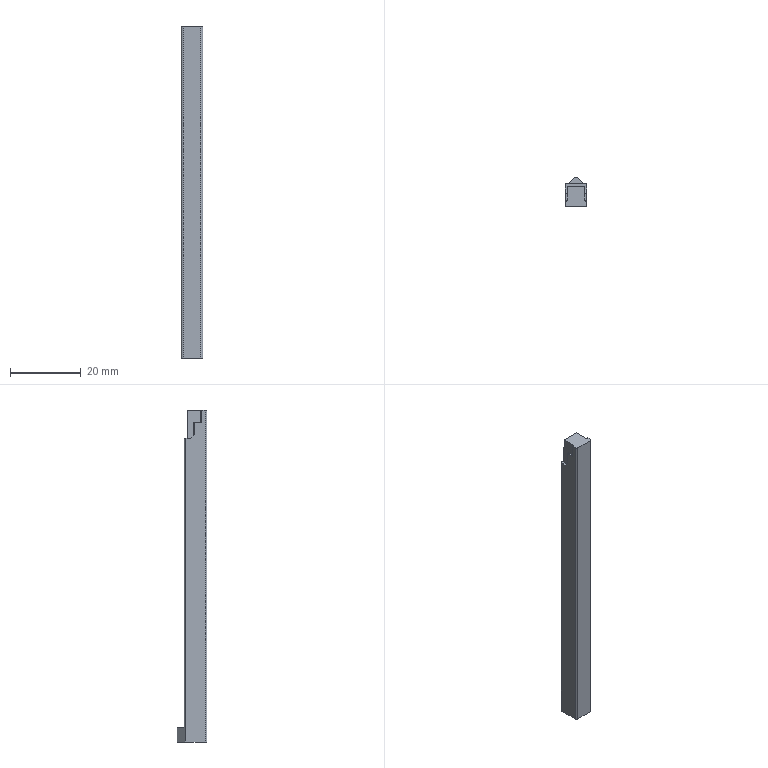Part | Creo | 1 solid | 30 faces | box 6.096 x 8.5 x 94.171 mm | volume 3667 mm3 | plane 22 | cylinder 8 | commonest cylinder face diameters 0.603 x4 1 x4
STEP:
#1=CARTESIAN_POINT('',(0.,0.,0.));
#2=DIRECTION('',(0.,0.,1.));
#3=DIRECTION('',(1.,0.,0.));
#4=AXIS2_PLACEMENT_3D('',#1,#2,#3);
#5=CARTESIAN_POINT('',(-2.088,17.979,36.563));
#6=VERTEX_POINT('',#5);
#7=CARTESIAN_POINT('',(-1.787,17.677,36.563));
#8=VERTEX_POINT('',#7);
#9=CARTESIAN_POINT('',(-2.088,17.878,36.563));
#10=CARTESIAN_POINT('',(-2.012,17.754,36.563));
#11=CARTESIAN_POINT('',(-1.887,17.677,36.563));
#12=B_SPLINE_CURVE_WITH_KNOTS('',3,(#5,#9,#10,#11,#7),.UNSPECIFIED.,.F.,.F.,(4,1,4),(0.,0.5,1.),.UNSPECIFIED.);
#13=EDGE_CURVE('',#6,#8,#12,.T.);
#14=ORIENTED_EDGE('',*,*,#13,.F.);
#15=CARTESIAN_POINT('',(-2.055,18.012,32.744));
#16=VERTEX_POINT('',#15);
#17=CARTESIAN_POINT('',(-2.088,17.979,36.563));
#18=DIRECTION('',(0.008726,0.008726,-0.9999));
#19=VECTOR('',#18,3.819);
#20=LINE('',#17,#19);
#21=EDGE_CURVE('',#6,#16,#20,.T.);
#22=ORIENTED_EDGE('',*,*,#21,.T.);
#23=CARTESIAN_POINT('',(-1.757,17.708,33.046));
#24=VERTEX_POINT('',#23);
#25=CARTESIAN_POINT('',(-1.757,17.708,33.046));
#26=CARTESIAN_POINT('',(-1.788,17.708,33.046));
#27=CARTESIAN_POINT('',(-1.849,17.718,33.036));
#28=CARTESIAN_POINT('',(-1.934,17.761,32.993));
#29=CARTESIAN_POINT('',(-1.999,17.826,32.929));
#30=CARTESIAN_POINT('',(-2.044,17.911,32.845));
#31=CARTESIAN_POINT('',(-2.055,17.977,32.78));
#32=B_SPLINE_CURVE_WITH_KNOTS('',3,(#25,#26,#27,#28,#29,#30,#31,#15),.UNSPECIFIED.,.F.,.F.,(4,1,1,1,1,4),(0.,0.2,0.4,0.6,0.8,1.),.UNSPECIFIED.);
#33=EDGE_CURVE('',#24,#16,#32,.T.);
#34=ORIENTED_EDGE('',*,*,#33,.F.);
#35=CARTESIAN_POINT('',(-1.757,17.708,33.046));
#36=DIRECTION('',(-0.008486,-0.008726,0.9999));
#37=VECTOR('',#36,3.518);
#38=LINE('',#35,#37);
#39=EDGE_CURVE('',#24,#8,#38,.T.);
#40=ORIENTED_EDGE('',*,*,#39,.T.);
#41=EDGE_LOOP('',(#14,#22,#34,#40));
#42=FACE_OUTER_BOUND('',#41,.F.);
#43=CARTESIAN_POINT('',(-0.6397,19.126,-94.88));
#44=DIRECTION('',(-0.008726,-0.008726,0.9999));
#45=DIRECTION('',(1.,0.,0.008727));
#46=AXIS2_PLACEMENT_3D('',#43,#44,#45);
#47=CYLINDRICAL_SURFACE('',#46,0.3015);
#48=ADVANCED_FACE('',(#42),#47,.F.);
#49=CARTESIAN_POINT('',(-1.553,15.668,36.563));
#50=VERTEX_POINT('',#49);
#51=CARTESIAN_POINT('',(-1.787,15.668,36.563));
#52=VERTEX_POINT('',#51);
#53=CARTESIAN_POINT('',(-1.553,15.668,36.563));
#54=DIRECTION('',(-1.,0.,0.));
#55=VECTOR('',#54,0.2342);
#56=LINE('',#53,#55);
#57=EDGE_CURVE('',#50,#52,#56,.T.);
#58=ORIENTED_EDGE('',*,*,#57,.T.);
#59=CARTESIAN_POINT('',(-2.088,15.969,36.563));
#60=VERTEX_POINT('',#59);
#61=CARTESIAN_POINT('',(-1.787,15.668,36.563));
#62=CARTESIAN_POINT('',(-1.887,15.668,36.563));
#63=CARTESIAN_POINT('',(-2.012,15.744,36.563));
#64=CARTESIAN_POINT('',(-2.088,15.868,36.563));
#65=CARTESIAN_POINT('',(-2.088,15.969,36.563));
#66=B_SPLINE_CURVE_WITH_KNOTS('',3,(#61,#62,#63,#64,#65),.UNSPECIFIED.,.F.,.F.,(4,1,4),(0.,0.5,1.),.UNSPECIFIED.);
#67=EDGE_CURVE('',#52,#60,#66,.T.);
#68=ORIENTED_EDGE('',*,*,#67,.T.);
#69=CARTESIAN_POINT('',(-2.088,17.979,36.563));
#70=DIRECTION('',(0.,-1.,0.));
#71=VECTOR('',#70,2.01);
#72=LINE('',#69,#71);
#73=EDGE_CURVE('',#6,#60,#72,.T.);
#74=ORIENTED_EDGE('',*,*,#73,.F.);
#75=ORIENTED_EDGE('',*,*,#13,.T.);
#76=CARTESIAN_POINT('',(-1.553,17.677,36.563));
#77=VERTEX_POINT('',#76);
#78=CARTESIAN_POINT('',(-1.553,17.677,36.563));
#79=DIRECTION('',(-1.,0.,0.));
#80=VECTOR('',#79,0.2342);
#81=LINE('',#78,#80);
#82=EDGE_CURVE('',#77,#8,#81,.T.);
#83=ORIENTED_EDGE('',*,*,#82,.F.);
#84=CARTESIAN_POINT('',(-1.553,17.677,36.563));
#85=DIRECTION('',(0.,-1.,0.));
#86=VECTOR('',#85,2.01);
#87=LINE('',#84,#86);
#88=EDGE_CURVE('',#77,#50,#87,.T.);
#89=ORIENTED_EDGE('',*,*,#88,.T.);
#90=EDGE_LOOP('',(#58,#68,#74,#75,#83,#89));
#91=FACE_OUTER_BOUND('',#90,.F.);
#92=CARTESIAN_POINT('',(-0.07825,-88.35,36.563));
#93=DIRECTION('',(0.,0.,1.));
#94=DIRECTION('',(0.,-1.,0.));
#95=AXIS2_PLACEMENT_3D('',#92,#93,#94);
#96=PLANE('',#95);
#97=ADVANCED_FACE('',(#91),#96,.T.);
#98=CARTESIAN_POINT('',(-1.553,15.637,40.081));
#99=VERTEX_POINT('',#98);
#100=CARTESIAN_POINT('',(-1.553,15.668,36.563));
#101=DIRECTION('',(0.,-0.008727,1.));
#102=VECTOR('',#101,3.518);
#103=LINE('',#100,#102);
#104=EDGE_CURVE('',#50,#99,#103,.T.);
#105=ORIENTED_EDGE('',*,*,#104,.T.);
#106=CARTESIAN_POINT('',(-1.817,15.637,40.081));
#107=VERTEX_POINT('',#106);
#108=CARTESIAN_POINT('',(-1.553,15.637,40.081));
#109=DIRECTION('',(-1.,0.,0.));
#110=VECTOR('',#109,0.2649);
#111=LINE('',#108,#110);
#112=EDGE_CURVE('',#99,#107,#111,.T.);
#113=ORIENTED_EDGE('',*,*,#112,.T.);
#114=CARTESIAN_POINT('',(-1.787,15.668,36.563));
#115=DIRECTION('',(-0.008726,-0.008726,0.9999));
#116=VECTOR('',#115,3.518);
#117=LINE('',#114,#116);
#118=EDGE_CURVE('',#52,#107,#117,.T.);
#119=ORIENTED_EDGE('',*,*,#118,.F.);
#120=ORIENTED_EDGE('',*,*,#57,.F.);
#121=EDGE_LOOP('',(#105,#113,#119,#120));
#122=FACE_OUTER_BOUND('',#121,.F.);
#123=CARTESIAN_POINT('',(1.526,15.668,36.563));
#124=DIRECTION('',(0.,-1.,-0.008727));
#125=DIRECTION('',(1.,0.,0.));
#126=AXIS2_PLACEMENT_3D('',#123,#124,#125);
#127=PLANE('',#126);
#128=ADVANCED_FACE('',(#122),#127,.F.);
#129=CARTESIAN_POINT('',(-1.553,20.123,32.041));
#130=VERTEX_POINT('',#129);
#131=CARTESIAN_POINT('',(-1.553,20.123,-54.09));
#132=VERTEX_POINT('',#131);
#133=CARTESIAN_POINT('',(-1.553,20.123,32.041));
#134=DIRECTION('',(0.,0.,-1.));
#135=VECTOR('',#134,86.131);
#136=LINE('',#133,#135);
#137=EDGE_CURVE('',#130,#132,#136,.T.);
#138=ORIENTED_EDGE('',*,*,#137,.T.);
#139=CARTESIAN_POINT('',(-1.553,14.623,-54.09));
#140=VERTEX_POINT('',#139);
#141=CARTESIAN_POINT('',(-1.553,20.123,-54.09));
#142=DIRECTION('',(0.,-1.,0.));
#143=VECTOR('',#142,5.5);
#144=LINE('',#141,#143);
#145=EDGE_CURVE('',#132,#140,#144,.T.);
#146=ORIENTED_EDGE('',*,*,#145,.T.);
#147=CARTESIAN_POINT('',(-1.553,14.623,40.081));
#148=VERTEX_POINT('',#147);
#149=CARTESIAN_POINT('',(-1.553,14.623,-54.09));
#150=DIRECTION('',(0.,0.,1.));
#151=VECTOR('',#150,94.171);
#152=LINE('',#149,#151);
#153=EDGE_CURVE('',#140,#148,#152,.T.);
#154=ORIENTED_EDGE('',*,*,#153,.T.);
#155=CARTESIAN_POINT('',(-1.553,15.637,40.081));
#156=DIRECTION('',(0.,-1.,0.));
#157=VECTOR('',#156,1.014);
#158=LINE('',#155,#157);
#159=EDGE_CURVE('',#99,#148,#158,.T.);
#160=ORIENTED_EDGE('',*,*,#159,.F.);
#161=ORIENTED_EDGE('',*,*,#104,.F.);
#162=ORIENTED_EDGE('',*,*,#88,.F.);
#163=CARTESIAN_POINT('',(-1.553,17.708,33.046));
#164=VERTEX_POINT('',#163);
#165=CARTESIAN_POINT('',(-1.553,17.708,33.046));
#166=DIRECTION('',(0.,-0.008727,1.));
#167=VECTOR('',#166,3.518);
#168=LINE('',#165,#167);
#169=EDGE_CURVE('',#164,#77,#168,.T.);
#170=ORIENTED_EDGE('',*,*,#169,.F.);
#171=CARTESIAN_POINT('',(-1.553,18.722,32.041));
#172=VERTEX_POINT('',#171);
#173=CARTESIAN_POINT('',(-1.553,18.722,32.041));
#174=DIRECTION('',(0.,-0.7102,0.704));
#175=VECTOR('',#174,1.427);
#176=LINE('',#173,#175);
#177=EDGE_CURVE('',#172,#164,#176,.T.);
#178=ORIENTED_EDGE('',*,*,#177,.F.);
#179=CARTESIAN_POINT('',(-1.553,18.722,32.041));
#180=DIRECTION('',(0.,1.,0.));
#181=VECTOR('',#180,1.401);
#182=LINE('',#179,#181);
#183=EDGE_CURVE('',#172,#130,#182,.T.);
#184=ORIENTED_EDGE('',*,*,#183,.T.);
#185=EDGE_LOOP('',(#138,#146,#154,#160,#161,#162,#170,#178,#184));
#186=FACE_OUTER_BOUND('',#185,.F.);
#187=CARTESIAN_POINT('',(-1.553,17.38,-97.959));
#188=DIRECTION('',(1.,0.,0.));
#189=DIRECTION('',(0.,0.,-1.));
#190=AXIS2_PLACEMENT_3D('',#187,#188,#189);
#191=PLANE('',#190);
#192=ADVANCED_FACE('',(#186),#191,.T.);
#193=CARTESIAN_POINT('',(-2.053,20.623,-50.09));
#194=VERTEX_POINT('',#193);
#195=CARTESIAN_POINT('',(-2.053,20.623,32.041));
#196=VERTEX_POINT('',#195);
#197=CARTESIAN_POINT('',(-2.053,20.623,-50.09));
#198=DIRECTION('',(0.,0.,1.));
#199=VECTOR('',#198,82.131);
#200=LINE('',#197,#199);
#201=EDGE_CURVE('',#194,#196,#200,.T.);
#202=ORIENTED_EDGE('',*,*,#201,.F.);
#203=CARTESIAN_POINT('',(-2.053,20.623,-54.09));
#204=VERTEX_POINT('',#203);
#205=CARTESIAN_POINT('',(-2.053,20.623,-54.09));
#206=DIRECTION('',(0.,0.,1.));
#207=VECTOR('',#206,4.);
#208=LINE('',#205,#207);
#209=EDGE_CURVE('',#204,#194,#208,.T.);
#210=ORIENTED_EDGE('',*,*,#209,.F.);
#211=CARTESIAN_POINT('',(-2.053,20.123,-54.09));
#212=DIRECTION('',(0.,0.,-1.));
#213=DIRECTION('',(0.,1.,0.));
#214=AXIS2_PLACEMENT_3D('',#211,#212,#213);
#215=CIRCLE('',#214,0.5);
#216=EDGE_CURVE('',#204,#132,#215,.T.);
#217=ORIENTED_EDGE('',*,*,#216,.T.);
#218=ORIENTED_EDGE('',*,*,#137,.F.);
#219=CARTESIAN_POINT('',(-2.053,20.123,32.041));
#220=DIRECTION('',(0.,0.,1.));
#221=DIRECTION('',(1.,0.,0.));
#222=AXIS2_PLACEMENT_3D('',#219,#220,#221);
#223=CIRCLE('',#222,0.5);
#224=EDGE_CURVE('',#130,#196,#223,.T.);
#225=ORIENTED_EDGE('',*,*,#224,.T.);
#226=EDGE_LOOP('',(#202,#210,#217,#218,#225));
#227=FACE_OUTER_BOUND('',#226,.F.);
#228=CARTESIAN_POINT('',(-2.053,20.123,-97.959));
#229=DIRECTION('',(0.,0.,1.));
#230=DIRECTION('',(1.,0.,0.));
#231=AXIS2_PLACEMENT_3D('',#228,#229,#230);
#232=CYLINDRICAL_SURFACE('',#231,0.5);
#233=ADVANCED_FACE('',(#227),#232,.T.);
#234=CARTESIAN_POINT('',(-7.149,20.623,-50.09));
#235=VERTEX_POINT('',#234);
#236=CARTESIAN_POINT('',(-2.053,20.623,-50.09));
#237=DIRECTION('',(-1.,0.,0.));
#238=VECTOR('',#237,5.096);
#239=LINE('',#236,#238);
#240=EDGE_CURVE('',#194,#235,#239,.T.);
#241=ORIENTED_EDGE('',*,*,#240,.F.);
#242=ORIENTED_EDGE('',*,*,#201,.T.);
#243=CARTESIAN_POINT('',(-7.149,20.623,32.041));
#244=VERTEX_POINT('',#243);
#245=CARTESIAN_POINT('',(-2.053,20.623,32.041));
#246=DIRECTION('',(-1.,0.,0.));
#247=VECTOR('',#246,5.096);
#248=LINE('',#245,#247);
#249=EDGE_CURVE('',#196,#244,#248,.T.);
#250=ORIENTED_EDGE('',*,*,#249,.T.);
#251=CARTESIAN_POINT('',(-7.149,20.623,32.041));
#252=DIRECTION('',(0.,0.,-1.));
#253=VECTOR('',#252,82.131);
#254=LINE('',#251,#253);
#255=EDGE_CURVE('',#244,#235,#254,.T.);
#256=ORIENTED_EDGE('',*,*,#255,.T.);
#257=EDGE_LOOP('',(#241,#242,#250,#256));
#258=FACE_OUTER_BOUND('',#257,.F.);
#259=CARTESIAN_POINT('',(-4.601,20.623,-97.959));
#260=DIRECTION('',(0.,1.,0.));
#261=DIRECTION('',(0.,0.,1.));
#262=AXIS2_PLACEMENT_3D('',#259,#260,#261);
#263=PLANE('',#262);
#264=ADVANCED_FACE('',(#258),#263,.T.);
#265=ORIENTED_EDGE('',*,*,#240,.T.);
#266=CARTESIAN_POINT('',(-5.149,22.623,-50.09));
#267=VERTEX_POINT('',#266);
#268=CARTESIAN_POINT('',(-5.149,22.623,-50.09));
#269=DIRECTION('',(-0.7071,-0.7071,0.));
#270=VECTOR('',#269,2.828);
#271=LINE('',#268,#270);
#272=EDGE_CURVE('',#267,#235,#271,.T.);
#273=ORIENTED_EDGE('',*,*,#272,.F.);
#274=CARTESIAN_POINT('',(-4.053,22.623,-50.09));
#275=VERTEX_POINT('',#274);
#276=CARTESIAN_POINT('',(-4.053,22.623,-50.09));
#277=DIRECTION('',(-1.,0.,0.));
#278=VECTOR('',#277,1.096);
#279=LINE('',#276,#278);
#280=EDGE_CURVE('',#275,#267,#279,.T.);
#281=ORIENTED_EDGE('',*,*,#280,.F.);
#282=CARTESIAN_POINT('',(-2.053,20.623,-50.09));
#283=DIRECTION('',(-0.7071,0.7071,0.));
#284=VECTOR('',#283,2.828);
#285=LINE('',#282,#284);
#286=EDGE_CURVE('',#194,#275,#285,.T.);
#287=ORIENTED_EDGE('',*,*,#286,.F.);
#288=EDGE_LOOP('',(#265,#273,#281,#287));
#289=FACE_OUTER_BOUND('',#288,.F.);
#290=CARTESIAN_POINT('',(-4.601,21.123,-50.09));
#291=DIRECTION('',(0.,0.,1.));
#292=DIRECTION('',(1.,0.,0.));
#293=AXIS2_PLACEMENT_3D('',#290,#291,#292);
#294=PLANE('',#293);
#295=ADVANCED_FACE('',(#289),#294,.T.);
#296=CARTESIAN_POINT('',(-7.149,20.623,-54.09));
#297=VERTEX_POINT('',#296);
#298=CARTESIAN_POINT('',(-5.149,22.623,-54.09));
#299=VERTEX_POINT('',#298);
#300=CARTESIAN_POINT('',(-7.149,20.623,-54.09));
#301=DIRECTION('',(0.7071,0.7071,0.));
#302=VECTOR('',#301,2.828);
#303=LINE('',#300,#302);
#304=EDGE_CURVE('',#297,#299,#303,.T.);
#305=ORIENTED_EDGE('',*,*,#304,.T.);
#306=CARTESIAN_POINT('',(-5.149,22.623,-50.09));
#307=DIRECTION('',(0.,0.,-1.));
#308=VECTOR('',#307,4.);
#309=LINE('',#306,#308);
#310=EDGE_CURVE('',#267,#299,#309,.T.);
#311=ORIENTED_EDGE('',*,*,#310,.F.);
#312=ORIENTED_EDGE('',*,*,#272,.T.);
#313=CARTESIAN_POINT('',(-7.149,20.623,-50.09));
#314=DIRECTION('',(0.,0.,-1.));
#315=VECTOR('',#314,4.);
#316=LINE('',#313,#315);
#317=EDGE_CURVE('',#235,#297,#316,.T.);
#318=ORIENTED_EDGE('',*,*,#317,.T.);
#319=EDGE_LOOP('',(#305,#311,#312,#318));
#320=FACE_OUTER_BOUND('',#319,.F.);
#321=CARTESIAN_POINT('',(-5.149,22.623,-54.09));
#322=DIRECTION('',(0.7071,-0.7071,0.));
#323=DIRECTION('',(0.,0.,1.));
#324=AXIS2_PLACEMENT_3D('',#321,#322,#323);
#325=PLANE('',#324);
#326=ADVANCED_FACE('',(#320),#325,.F.);
#327=CARTESIAN_POINT('',(-4.053,22.623,-54.09));
#328=VERTEX_POINT('',#327);
#329=CARTESIAN_POINT('',(-5.149,22.623,-54.09));
#330=DIRECTION('',(1.,0.,0.));
#331=VECTOR('',#330,1.096);
#332=LINE('',#329,#331);
#333=EDGE_CURVE('',#299,#328,#332,.T.);
#334=ORIENTED_EDGE('',*,*,#333,.F.);
#335=ORIENTED_EDGE('',*,*,#304,.F.);
#336=CARTESIAN_POINT('',(-7.649,20.123,-54.09));
#337=VERTEX_POINT('',#336);
#338=CARTESIAN_POINT('',(-7.149,20.123,-54.09));
#339=DIRECTION('',(0.,0.,-1.));
#340=DIRECTION('',(-1.,0.,0.));
#341=AXIS2_PLACEMENT_3D('',#338,#339,#340);
#342=CIRCLE('',#341,0.5);
#343=EDGE_CURVE('',#337,#297,#342,.T.);
#344=ORIENTED_EDGE('',*,*,#343,.F.);
#345=CARTESIAN_POINT('',(-7.649,14.623,-54.09));
#346=VERTEX_POINT('',#345);
#347=CARTESIAN_POINT('',(-7.649,14.623,-54.09));
#348=DIRECTION('',(0.,1.,0.));
#349=VECTOR('',#348,5.5);
#350=LINE('',#347,#349);
#351=EDGE_CURVE('',#346,#337,#350,.T.);
#352=ORIENTED_EDGE('',*,*,#351,.F.);
#353=CARTESIAN_POINT('',(-7.149,14.123,-54.09));
#354=VERTEX_POINT('',#353);
#355=CARTESIAN_POINT('',(-7.149,14.623,-54.09));
#356=DIRECTION('',(0.,0.,-1.));
#357=DIRECTION('',(0.,-1.,0.));
#358=AXIS2_PLACEMENT_3D('',#355,#356,#357);
#359=CIRCLE('',#358,0.5);
#360=EDGE_CURVE('',#354,#346,#359,.T.);
#361=ORIENTED_EDGE('',*,*,#360,.F.);
#362=CARTESIAN_POINT('',(-2.053,14.123,-54.09));
#363=VERTEX_POINT('',#362);
#364=CARTESIAN_POINT('',(-2.053,14.123,-54.09));
#365=DIRECTION('',(-1.,0.,0.));
#366=VECTOR('',#365,5.096);
#367=LINE('',#364,#366);
#368=EDGE_CURVE('',#363,#354,#367,.T.);
#369=ORIENTED_EDGE('',*,*,#368,.F.);
#370=CARTESIAN_POINT('',(-2.053,14.623,-54.09));
#371=DIRECTION('',(0.,0.,-1.));
#372=DIRECTION('',(1.,0.,0.));
#373=AXIS2_PLACEMENT_3D('',#370,#371,#372);
#374=CIRCLE('',#373,0.5);
#375=EDGE_CURVE('',#140,#363,#374,.T.);
#376=ORIENTED_EDGE('',*,*,#375,.F.);
#377=ORIENTED_EDGE('',*,*,#145,.F.);
#378=ORIENTED_EDGE('',*,*,#216,.F.);
#379=CARTESIAN_POINT('',(-4.053,22.623,-54.09));
#380=DIRECTION('',(0.7071,-0.7071,0.));
#381=VECTOR('',#380,2.828);
#382=LINE('',#379,#381);
#383=EDGE_CURVE('',#328,#204,#382,.T.);
#384=ORIENTED_EDGE('',*,*,#383,.F.);
#385=EDGE_LOOP('',(#334,#335,#344,#352,#361,#369,#376,#377,#378,#384));
#386=FACE_OUTER_BOUND('',#385,.F.);
#387=CARTESIAN_POINT('',(0.,0.,-54.09));
#388=DIRECTION('',(0.,0.,-1.));
#389=DIRECTION('',(-1.,0.,0.));
#390=AXIS2_PLACEMENT_3D('',#387,#388,#389);
#391=PLANE('',#390);
#392=ADVANCED_FACE('',(#386),#391,.T.);
#393=ORIENTED_EDGE('',*,*,#280,.T.);
#394=ORIENTED_EDGE('',*,*,#310,.T.);
#395=ORIENTED_EDGE('',*,*,#333,.T.);
#396=CARTESIAN_POINT('',(-4.053,22.623,-54.09));
#397=DIRECTION('',(0.,0.,1.));
#398=VECTOR('',#397,4.);
#399=LINE('',#396,#398);
#400=EDGE_CURVE('',#328,#275,#399,.T.);
#401=ORIENTED_EDGE('',*,*,#400,.T.);
#402=EDGE_LOOP('',(#393,#394,#395,#401));
#403=FACE_OUTER_BOUND('',#402,.F.);
#404=CARTESIAN_POINT('',(-4.601,22.623,-54.09));
#405=DIRECTION('',(0.,1.,0.));
#406=DIRECTION('',(0.,0.,1.));
#407=AXIS2_PLACEMENT_3D('',#404,#405,#406);
#408=PLANE('',#407);
#409=ADVANCED_FACE('',(#403),#408,.T.);
#410=ORIENTED_EDGE('',*,*,#383,.T.);
#411=ORIENTED_EDGE('',*,*,#209,.T.);
#412=ORIENTED_EDGE('',*,*,#286,.T.);
#413=ORIENTED_EDGE('',*,*,#400,.F.);
#414=EDGE_LOOP('',(#410,#411,#412,#413));
#415=FACE_OUTER_BOUND('',#414,.F.);
#416=CARTESIAN_POINT('',(-2.053,20.623,-54.09));
#417=DIRECTION('',(-0.7071,-0.7071,0.));
#418=DIRECTION('',(0.,0.,1.));
#419=AXIS2_PLACEMENT_3D('',#416,#417,#418);
#420=PLANE('',#419);
#421=ADVANCED_FACE('',(#415),#420,.F.);
#422=CARTESIAN_POINT('',(-7.649,20.123,32.041));
#423=VERTEX_POINT('',#422);
#424=CARTESIAN_POINT('',(-7.649,20.123,-54.09));
#425=DIRECTION('',(0.,0.,1.));
#426=VECTOR('',#425,86.131);
#427=LINE('',#424,#426);
#428=EDGE_CURVE('',#337,#423,#427,.T.);
#429=ORIENTED_EDGE('',*,*,#428,.F.);
#430=ORIENTED_EDGE('',*,*,#343,.T.);
#431=ORIENTED_EDGE('',*,*,#317,.F.);
#432=ORIENTED_EDGE('',*,*,#255,.F.);
#433=CARTESIAN_POINT('',(-7.149,20.123,32.041));
#434=DIRECTION('',(0.,0.,1.));
#435=DIRECTION('',(0.,1.,0.));
#436=AXIS2_PLACEMENT_3D('',#433,#434,#435);
#437=CIRCLE('',#436,0.5);
#438=EDGE_CURVE('',#244,#423,#437,.T.);
#439=ORIENTED_EDGE('',*,*,#438,.T.);
#440=EDGE_LOOP('',(#429,#430,#431,#432,#439));
#441=FACE_OUTER_BOUND('',#440,.F.);
#442=CARTESIAN_POINT('',(-7.149,20.123,-97.959));
#443=DIRECTION('',(0.,0.,1.));
#444=DIRECTION('',(1.,0.,0.));
#445=AXIS2_PLACEMENT_3D('',#442,#443,#444);
#446=CYLINDRICAL_SURFACE('',#445,0.5);
#447=ADVANCED_FACE('',(#441),#446,.T.);
#448=CARTESIAN_POINT('',(-7.649,17.708,33.046));
#449=VERTEX_POINT('',#448);
#450=CARTESIAN_POINT('',(-7.649,18.722,32.041));
#451=VERTEX_POINT('',#450);
#452=CARTESIAN_POINT('',(-7.649,17.708,33.046));
#453=DIRECTION('',(0.,0.7102,-0.704));
#454=VECTOR('',#453,1.427);
#455=LINE('',#452,#454);
#456=EDGE_CURVE('',#449,#451,#455,.T.);
#457=ORIENTED_EDGE('',*,*,#456,.F.);
#458=CARTESIAN_POINT('',(-7.649,17.677,36.563));
#459=VERTEX_POINT('',#458);
#460=CARTESIAN_POINT('',(-7.649,17.677,36.563));
#461=DIRECTION('',(0.,0.008727,-1.));
#462=VECTOR('',#461,3.518);
#463=LINE('',#460,#462);
#464=EDGE_CURVE('',#459,#449,#463,.T.);
#465=ORIENTED_EDGE('',*,*,#464,.F.);
#466=CARTESIAN_POINT('',(-7.649,15.668,36.563));
#467=VERTEX_POINT('',#466);
#468=CARTESIAN_POINT('',(-7.649,15.668,36.563));
#469=DIRECTION('',(0.,1.,0.));
#470=VECTOR('',#469,2.01);
#471=LINE('',#468,#470);
#472=EDGE_CURVE('',#467,#459,#471,.T.);
#473=ORIENTED_EDGE('',*,*,#472,.F.);
#474=CARTESIAN_POINT('',(-7.649,15.637,40.081));
#475=VERTEX_POINT('',#474);
#476=CARTESIAN_POINT('',(-7.649,15.637,40.081));
#477=DIRECTION('',(0.,0.008727,-1.));
#478=VECTOR('',#477,3.518);
#479=LINE('',#476,#478);
#480=EDGE_CURVE('',#475,#467,#479,.T.);
#481=ORIENTED_EDGE('',*,*,#480,.F.);
#482=CARTESIAN_POINT('',(-7.649,14.623,40.081));
#483=VERTEX_POINT('',#482);
#484=CARTESIAN_POINT('',(-7.649,14.623,40.081));
#485=DIRECTION('',(0.,1.,0.));
#486=VECTOR('',#485,1.014);
#487=LINE('',#484,#486);
#488=EDGE_CURVE('',#483,#475,#487,.T.);
#489=ORIENTED_EDGE('',*,*,#488,.F.);
#490=CARTESIAN_POINT('',(-7.649,14.623,40.081));
#491=DIRECTION('',(0.,0.,-1.));
#492=VECTOR('',#491,94.171);
#493=LINE('',#490,#492);
#494=EDGE_CURVE('',#483,#346,#493,.T.);
#495=ORIENTED_EDGE('',*,*,#494,.T.);
#496=ORIENTED_EDGE('',*,*,#351,.T.);
#497=ORIENTED_EDGE('',*,*,#428,.T.);
#498=CARTESIAN_POINT('',(-7.649,20.123,32.041));
#499=DIRECTION('',(0.,-1.,0.));
#500=VECTOR('',#499,1.401);
#501=LINE('',#498,#500);
#502=EDGE_CURVE('',#423,#451,#501,.T.);
#503=ORIENTED_EDGE('',*,*,#502,.T.);
#504=EDGE_LOOP('',(#457,#465,#473,#481,#489,#495,#496,#497,#503));
#505=FACE_OUTER_BOUND('',#504,.F.);
#506=CARTESIAN_POINT('',(-7.649,17.38,-97.959));
#507=DIRECTION('',(-1.,0.,0.));
#508=DIRECTION('',(0.,0.,1.));
#509=AXIS2_PLACEMENT_3D('',#506,#507,#508);
#510=PLANE('',#509);
#511=ADVANCED_FACE('',(#505),#510,.T.);
#512=ORIENTED_EDGE('',*,*,#456,.T.);
#513=CARTESIAN_POINT('',(-7.153,18.722,32.041));
#514=VERTEX_POINT('',#513);
#515=CARTESIAN_POINT('',(-7.153,18.722,32.041));
#516=DIRECTION('',(-1.,0.,0.));
#517=VECTOR('',#516,0.4962);
#518=LINE('',#515,#517);
#519=EDGE_CURVE('',#514,#451,#518,.T.);
#520=ORIENTED_EDGE('',*,*,#519,.F.);
#521=CARTESIAN_POINT('',(-7.147,18.012,32.744));
#522=VERTEX_POINT('',#521);
#523=CARTESIAN_POINT('',(-7.153,18.722,32.041));
#524=DIRECTION('',(0.006144,-0.7102,0.704));
#525=VECTOR('',#524,0.9993);
#526=LINE('',#523,#525);
#527=EDGE_CURVE('',#514,#522,#526,.T.);
#528=ORIENTED_EDGE('',*,*,#527,.T.);
#529=CARTESIAN_POINT('',(-7.445,17.708,33.046));
#530=VERTEX_POINT('',#529);
#531=CARTESIAN_POINT('',(-7.147,18.012,32.744));
#532=CARTESIAN_POINT('',(-7.146,17.977,32.78));
#533=CARTESIAN_POINT('',(-7.157,17.911,32.845));
#534=CARTESIAN_POINT('',(-7.202,17.826,32.929));
#535=CARTESIAN_POINT('',(-7.268,17.761,32.994));
#536=CARTESIAN_POINT('',(-7.354,17.717,33.037));
#537=CARTESIAN_POINT('',(-7.414,17.708,33.046));
#538=B_SPLINE_CURVE_WITH_KNOTS('',3,(#531,#532,#533,#534,#535,#536,#537,#529),.UNSPECIFIED.,.F.,.F.,(4,1,1,1,1,4),(0.,0.2,0.4,0.6,0.8,1.),.UNSPECIFIED.);
#539=EDGE_CURVE('',#522,#530,#538,.T.);
#540=ORIENTED_EDGE('',*,*,#539,.T.);
#541=CARTESIAN_POINT('',(-7.445,17.708,33.046));
#542=DIRECTION('',(-1.,0.000005682,-0.0006511));
#543=VECTOR('',#542,0.2044);
#544=LINE('',#541,#543);
#545=EDGE_CURVE('',#530,#449,#544,.T.);
#546=ORIENTED_EDGE('',*,*,#545,.T.);
#547=EDGE_LOOP('',(#512,#520,#528,#540,#546));
#548=FACE_OUTER_BOUND('',#547,.F.);
#549=CARTESIAN_POINT('',(-7.616,18.215,32.543));
#550=DIRECTION('',(0.,-0.704,-0.7102));
#551=DIRECTION('',(0.,0.7102,-0.704));
#552=AXIS2_PLACEMENT_3D('',#549,#550,#551);
#553=PLANE('',#552);
#554=ADVANCED_FACE('',(#548),#553,.F.);
#555=ORIENTED_EDGE('',*,*,#502,.F.);
#556=ORIENTED_EDGE('',*,*,#438,.F.);
#557=ORIENTED_EDGE('',*,*,#249,.F.);
#558=ORIENTED_EDGE('',*,*,#224,.F.);
#559=ORIENTED_EDGE('',*,*,#183,.F.);
#560=CARTESIAN_POINT('',(-2.049,18.722,32.041));
#561=VERTEX_POINT('',#560);
#562=CARTESIAN_POINT('',(-1.553,18.722,32.041));
#563=DIRECTION('',(-1.,0.,0.));
#564=VECTOR('',#563,0.4962);
#565=LINE('',#562,#564);
#566=EDGE_CURVE('',#172,#561,#565,.T.);
#567=ORIENTED_EDGE('',*,*,#566,.T.);
#568=CARTESIAN_POINT('',(-2.049,19.727,32.041));
#569=VERTEX_POINT('',#568);
#570=CARTESIAN_POINT('',(-2.049,18.722,32.041));
#571=DIRECTION('',(0.,1.,0.));
#572=VECTOR('',#571,1.005);
#573=LINE('',#570,#572);
#574=EDGE_CURVE('',#561,#569,#573,.T.);
#575=ORIENTED_EDGE('',*,*,#574,.T.);
#576=CARTESIAN_POINT('',(-7.153,19.727,32.041));
#577=VERTEX_POINT('',#576);
#578=CARTESIAN_POINT('',(-2.049,19.727,32.041));
#579=DIRECTION('',(-1.,0.,0.));
#580=VECTOR('',#579,5.104);
#581=LINE('',#578,#580);
#582=EDGE_CURVE('',#569,#577,#581,.T.);
#583=ORIENTED_EDGE('',*,*,#582,.T.);
#584=CARTESIAN_POINT('',(-7.153,19.727,32.041));
#585=DIRECTION('',(0.,-1.,0.));
#586=VECTOR('',#585,1.005);
#587=LINE('',#584,#586);
#588=EDGE_CURVE('',#577,#514,#587,.T.);
#589=ORIENTED_EDGE('',*,*,#588,.T.);
#590=ORIENTED_EDGE('',*,*,#519,.T.);
#591=EDGE_LOOP('',(#555,#556,#557,#558,#559,#567,#575,#583,#589,#590));
#592=FACE_OUTER_BOUND('',#591,.F.);
#593=CARTESIAN_POINT('',(-0.07825,-88.35,32.041));
#594=DIRECTION('',(0.,0.,-1.));
#595=DIRECTION('',(0.,-1.,0.));
#596=AXIS2_PLACEMENT_3D('',#593,#594,#595);
#597=PLANE('',#596);
#598=ADVANCED_FACE('',(#592),#597,.F.);
#599=ORIENTED_EDGE('',*,*,#177,.T.);
#600=CARTESIAN_POINT('',(-1.553,17.708,33.046));
#601=DIRECTION('',(-1.,-0.00000575,0.0006588));
#602=VECTOR('',#601,0.2044);
#603=LINE('',#600,#602);
#604=EDGE_CURVE('',#164,#24,#603,.T.);
#605=ORIENTED_EDGE('',*,*,#604,.T.);
#606=ORIENTED_EDGE('',*,*,#33,.T.);
#607=CARTESIAN_POINT('',(-2.055,18.012,32.744));
#608=DIRECTION('',(0.006144,0.7102,-0.704));
#609=VECTOR('',#608,0.9993);
#610=LINE('',#607,#609);
#611=EDGE_CURVE('',#16,#561,#610,.T.);
#612=ORIENTED_EDGE('',*,*,#611,.T.);
#613=ORIENTED_EDGE('',*,*,#566,.F.);
#614=EDGE_LOOP('',(#599,#605,#606,#612,#613));
#615=FACE_OUTER_BOUND('',#614,.F.);
#616=CARTESIAN_POINT('',(-1.586,18.215,32.543));
#617=DIRECTION('',(0.,-0.704,-0.7102));
#618=DIRECTION('',(0.,0.7102,-0.704));
#619=AXIS2_PLACEMENT_3D('',#616,#617,#618);
#620=PLANE('',#619);
#621=ADVANCED_FACE('',(#615),#620,.F.);
#622=ORIENTED_EDGE('',*,*,#169,.T.);
#623=ORIENTED_EDGE('',*,*,#82,.T.);
#624=ORIENTED_EDGE('',*,*,#39,.F.);
#625=ORIENTED_EDGE('',*,*,#604,.F.);
#626=EDGE_LOOP('',(#622,#623,#624,#625));
#627=FACE_OUTER_BOUND('',#626,.F.);
#628=CARTESIAN_POINT('',(1.526,17.677,36.563));
#629=DIRECTION('',(0.,-1.,-0.008727));
#630=DIRECTION('',(1.,0.,0.));
#631=AXIS2_PLACEMENT_3D('',#628,#629,#630);
#632=PLANE('',#631);
#633=ADVANCED_FACE('',(#627),#632,.F.);
#634=ORIENTED_EDGE('',*,*,#73,.T.);
#635=CARTESIAN_POINT('',(-2.119,15.938,40.081));
#636=VERTEX_POINT('',#635);
#637=CARTESIAN_POINT('',(-2.119,15.938,40.081));
#638=DIRECTION('',(0.008726,0.008726,-0.9999));
#639=VECTOR('',#638,3.518);
#640=LINE('',#637,#639);
#641=EDGE_CURVE('',#636,#60,#640,.T.);
#642=ORIENTED_EDGE('',*,*,#641,.F.);
#643=CARTESIAN_POINT('',(-2.119,19.657,40.081));
#644=VERTEX_POINT('',#643);
#645=CARTESIAN_POINT('',(-2.119,19.657,40.081));
#646=DIRECTION('',(0.,-1.,0.));
#647=VECTOR('',#646,3.719);
#648=LINE('',#645,#647);
#649=EDGE_CURVE('',#644,#636,#648,.T.);
#650=ORIENTED_EDGE('',*,*,#649,.F.);
#651=CARTESIAN_POINT('',(-2.119,19.657,40.081));
#652=DIRECTION('',(0.008726,0.008726,-0.9999));
#653=VECTOR('',#652,8.041);
#654=LINE('',#651,#653);
#655=EDGE_CURVE('',#644,#569,#654,.T.);
#656=ORIENTED_EDGE('',*,*,#655,.T.);
#657=ORIENTED_EDGE('',*,*,#574,.F.);
#658=ORIENTED_EDGE('',*,*,#611,.F.);
#659=ORIENTED_EDGE('',*,*,#21,.F.);
#660=EDGE_LOOP('',(#634,#642,#650,#656,#657,#658,#659));
#661=FACE_OUTER_BOUND('',#660,.F.);
#662=CARTESIAN_POINT('',(-2.088,13.058,36.563));
#663=DIRECTION('',(-1.,0.,-0.008727));
#664=DIRECTION('',(0.,-1.,0.));
#665=AXIS2_PLACEMENT_3D('',#662,#663,#664);
#666=PLANE('',#665);
#667=ADVANCED_FACE('',(#661),#666,.F.);
#668=CARTESIAN_POINT('',(-2.119,15.938,40.081));
#669=CARTESIAN_POINT('',(-2.119,15.838,40.081));
#670=CARTESIAN_POINT('',(-2.043,15.713,40.081));
#671=CARTESIAN_POINT('',(-1.918,15.637,40.081));
#672=B_SPLINE_CURVE_WITH_KNOTS('',3,(#668,#669,#670,#671,#106),.UNSPECIFIED.,.F.,.F.,(4,1,4),(0.,0.5,1.),.UNSPECIFIED.);
#673=EDGE_CURVE('',#636,#107,#672,.T.);
#674=ORIENTED_EDGE('',*,*,#673,.F.);
#675=ORIENTED_EDGE('',*,*,#641,.T.);
#676=ORIENTED_EDGE('',*,*,#67,.F.);
#677=ORIENTED_EDGE('',*,*,#118,.T.);
#678=EDGE_LOOP('',(#674,#675,#676,#677));
#679=FACE_OUTER_BOUND('',#678,.F.);
#680=CARTESIAN_POINT('',(-0.6397,17.116,-94.88));
#681=DIRECTION('',(-0.008726,-0.008726,0.9999));
#682=DIRECTION('',(1.,0.,0.008727));
#683=AXIS2_PLACEMENT_3D('',#680,#681,#682);
#684=CYLINDRICAL_SURFACE('',#683,0.3015);
#685=ADVANCED_FACE('',(#679),#684,.F.);
#686=CARTESIAN_POINT('',(-2.053,14.123,40.081));
#687=VERTEX_POINT('',#686);
#688=CARTESIAN_POINT('',(-2.053,14.623,40.081));
#689=DIRECTION('',(0.,0.,1.));
#690=DIRECTION('',(0.,-1.,0.));
#691=AXIS2_PLACEMENT_3D('',#688,#689,#690);
#692=CIRCLE('',#691,0.5);
#693=EDGE_CURVE('',#687,#148,#692,.T.);
#694=ORIENTED_EDGE('',*,*,#693,.F.);
#695=CARTESIAN_POINT('',(-7.149,14.123,40.081));
#696=VERTEX_POINT('',#695);
#697=CARTESIAN_POINT('',(-2.053,14.123,40.081));
#698=DIRECTION('',(-1.,0.,0.));
#699=VECTOR('',#698,5.096);
#700=LINE('',#697,#699);
#701=EDGE_CURVE('',#687,#696,#700,.T.);
#702=ORIENTED_EDGE('',*,*,#701,.T.);
#703=CARTESIAN_POINT('',(-7.149,14.623,40.081));
#704=DIRECTION('',(0.,0.,1.));
#705=DIRECTION('',(-1.,0.,0.));
#706=AXIS2_PLACEMENT_3D('',#703,#704,#705);
#707=CIRCLE('',#706,0.5);
#708=EDGE_CURVE('',#483,#696,#707,.T.);
#709=ORIENTED_EDGE('',*,*,#708,.F.);
#710=ORIENTED_EDGE('',*,*,#488,.T.);
#711=CARTESIAN_POINT('',(-7.384,15.637,40.081));
#712=VERTEX_POINT('',#711);
#713=CARTESIAN_POINT('',(-7.384,15.637,40.081));
#714=DIRECTION('',(-1.,0.,0.));
#715=VECTOR('',#714,0.2649);
#716=LINE('',#713,#715);
#717=EDGE_CURVE('',#712,#475,#716,.T.);
#718=ORIENTED_EDGE('',*,*,#717,.F.);
#719=CARTESIAN_POINT('',(-7.083,15.938,40.081));
#720=VERTEX_POINT('',#719);
#721=CARTESIAN_POINT('',(-7.284,15.637,40.081));
#722=CARTESIAN_POINT('',(-7.159,15.713,40.081));
#723=CARTESIAN_POINT('',(-7.083,15.838,40.081));
#724=B_SPLINE_CURVE_WITH_KNOTS('',3,(#711,#721,#722,#723,#719),.UNSPECIFIED.,.F.,.F.,(4,1,4),(0.,0.5,1.),.UNSPECIFIED.);
#725=EDGE_CURVE('',#712,#720,#724,.T.);
#726=ORIENTED_EDGE('',*,*,#725,.T.);
#727=CARTESIAN_POINT('',(-7.083,19.657,40.081));
#728=VERTEX_POINT('',#727);
#729=CARTESIAN_POINT('',(-7.083,15.938,40.081));
#730=DIRECTION('',(0.,1.,0.));
#731=VECTOR('',#730,3.719);
#732=LINE('',#729,#731);
#733=EDGE_CURVE('',#720,#728,#732,.T.);
#734=ORIENTED_EDGE('',*,*,#733,.T.);
#735=CARTESIAN_POINT('',(-2.119,19.657,40.081));
#736=DIRECTION('',(-1.,0.,0.));
#737=VECTOR('',#736,4.964);
#738=LINE('',#735,#737);
#739=EDGE_CURVE('',#644,#728,#738,.T.);
#740=ORIENTED_EDGE('',*,*,#739,.F.);
#741=ORIENTED_EDGE('',*,*,#649,.T.);
#742=ORIENTED_EDGE('',*,*,#673,.T.);
#743=ORIENTED_EDGE('',*,*,#112,.F.);
#744=ORIENTED_EDGE('',*,*,#159,.T.);
#745=EDGE_LOOP('',(#694,#702,#709,#710,#718,#726,#734,#740,#741,#742,#743,#744));
#746=FACE_OUTER_BOUND('',#745,.F.);
#747=CARTESIAN_POINT('',(-17.817,-88.35,40.081));
#748=DIRECTION('',(0.,0.,1.));
#749=DIRECTION('',(-1.,0.,0.));
#750=AXIS2_PLACEMENT_3D('',#747,#748,#749);
#751=PLANE('',#750);
#752=ADVANCED_FACE('',(#746),#751,.T.);
#753=ORIENTED_EDGE('',*,*,#693,.T.);
#754=ORIENTED_EDGE('',*,*,#153,.F.);
#755=ORIENTED_EDGE('',*,*,#375,.T.);
#756=CARTESIAN_POINT('',(-2.053,14.123,40.081));
#757=DIRECTION('',(0.,0.,-1.));
#758=VECTOR('',#757,94.171);
#759=LINE('',#756,#758);
#760=EDGE_CURVE('',#687,#363,#759,.T.);
#761=ORIENTED_EDGE('',*,*,#760,.F.);
#762=EDGE_LOOP('',(#753,#754,#755,#761));
#763=FACE_OUTER_BOUND('',#762,.F.);
#764=CARTESIAN_POINT('',(-2.053,14.623,-97.959));
#765=DIRECTION('',(0.,0.,-1.));
#766=DIRECTION('',(-1.,0.,0.));
#767=AXIS2_PLACEMENT_3D('',#764,#765,#766);
#768=CYLINDRICAL_SURFACE('',#767,0.5);
#769=ADVANCED_FACE('',(#763),#768,.T.);
#770=ORIENTED_EDGE('',*,*,#701,.F.);
#771=ORIENTED_EDGE('',*,*,#760,.T.);
#772=ORIENTED_EDGE('',*,*,#368,.T.);
#773=CARTESIAN_POINT('',(-7.149,14.123,-54.09));
#774=DIRECTION('',(0.,0.,1.));
#775=VECTOR('',#774,94.171);
#776=LINE('',#773,#775);
#777=EDGE_CURVE('',#354,#696,#776,.T.);
#778=ORIENTED_EDGE('',*,*,#777,.T.);
#779=EDGE_LOOP('',(#770,#771,#772,#778));
#780=FACE_OUTER_BOUND('',#779,.F.);
#781=CARTESIAN_POINT('',(-4.601,14.123,-97.959));
#782=DIRECTION('',(0.,1.,0.));
#783=DIRECTION('',(0.,0.,1.));
#784=AXIS2_PLACEMENT_3D('',#781,#782,#783);
#785=PLANE('',#784);
#786=ADVANCED_FACE('',(#780),#785,.F.);
#787=ORIENTED_EDGE('',*,*,#708,.T.);
#788=ORIENTED_EDGE('',*,*,#777,.F.);
#789=ORIENTED_EDGE('',*,*,#360,.T.);
#790=ORIENTED_EDGE('',*,*,#494,.F.);
#791=EDGE_LOOP('',(#787,#788,#789,#790));
#792=FACE_OUTER_BOUND('',#791,.F.);
#793=CARTESIAN_POINT('',(-7.149,14.623,-97.959));
#794=DIRECTION('',(0.,0.,-1.));
#795=DIRECTION('',(-1.,0.,0.));
#796=AXIS2_PLACEMENT_3D('',#793,#794,#795);
#797=CYLINDRICAL_SURFACE('',#796,0.5);
#798=ADVANCED_FACE('',(#792),#797,.T.);
#799=ORIENTED_EDGE('',*,*,#480,.T.);
#800=CARTESIAN_POINT('',(-7.415,15.668,36.563));
#801=VERTEX_POINT('',#800);
#802=CARTESIAN_POINT('',(-7.415,15.668,36.563));
#803=DIRECTION('',(-1.,0.,0.));
#804=VECTOR('',#803,0.2342);
#805=LINE('',#802,#804);
#806=EDGE_CURVE('',#801,#467,#805,.T.);
#807=ORIENTED_EDGE('',*,*,#806,.F.);
#808=CARTESIAN_POINT('',(-7.384,15.637,40.081));
#809=DIRECTION('',(-0.008726,0.008726,-0.9999));
#810=VECTOR('',#809,3.518);
#811=LINE('',#808,#810);
#812=EDGE_CURVE('',#712,#801,#811,.T.);
#813=ORIENTED_EDGE('',*,*,#812,.F.);
#814=ORIENTED_EDGE('',*,*,#717,.T.);
#815=EDGE_LOOP('',(#799,#807,#813,#814));
#816=FACE_OUTER_BOUND('',#815,.F.);
#817=CARTESIAN_POINT('',(-4.504,15.668,36.563));
#818=DIRECTION('',(0.,-1.,-0.008727));
#819=DIRECTION('',(1.,0.,0.));
#820=AXIS2_PLACEMENT_3D('',#817,#818,#819);
#821=PLANE('',#820);
#822=ADVANCED_FACE('',(#816),#821,.F.);
#823=CARTESIAN_POINT('',(-7.415,17.677,36.563));
#824=VERTEX_POINT('',#823);
#825=CARTESIAN_POINT('',(-7.415,17.677,36.563));
#826=DIRECTION('',(-1.,0.,0.));
#827=VECTOR('',#826,0.2342);
#828=LINE('',#825,#827);
#829=EDGE_CURVE('',#824,#459,#828,.T.);
#830=ORIENTED_EDGE('',*,*,#829,.F.);
#831=CARTESIAN_POINT('',(-7.113,17.979,36.563));
#832=VERTEX_POINT('',#831);
#833=CARTESIAN_POINT('',(-7.314,17.677,36.563));
#834=CARTESIAN_POINT('',(-7.189,17.754,36.563));
#835=CARTESIAN_POINT('',(-7.113,17.878,36.563));
#836=B_SPLINE_CURVE_WITH_KNOTS('',3,(#823,#833,#834,#835,#831),.UNSPECIFIED.,.F.,.F.,(4,1,4),(0.,0.5,1.),.UNSPECIFIED.);
#837=EDGE_CURVE('',#824,#832,#836,.T.);
#838=ORIENTED_EDGE('',*,*,#837,.T.);
#839=CARTESIAN_POINT('',(-7.113,15.969,36.563));
#840=VERTEX_POINT('',#839);
#841=CARTESIAN_POINT('',(-7.113,15.969,36.563));
#842=DIRECTION('',(0.,1.,0.));
#843=VECTOR('',#842,2.01);
#844=LINE('',#841,#843);
#845=EDGE_CURVE('',#840,#832,#844,.T.);
#846=ORIENTED_EDGE('',*,*,#845,.F.);
#847=CARTESIAN_POINT('',(-7.113,15.969,36.563));
#848=CARTESIAN_POINT('',(-7.113,15.868,36.563));
#849=CARTESIAN_POINT('',(-7.189,15.744,36.563));
#850=CARTESIAN_POINT('',(-7.314,15.668,36.563));
#851=B_SPLINE_CURVE_WITH_KNOTS('',3,(#847,#848,#849,#850,#800),.UNSPECIFIED.,.F.,.F.,(4,1,4),(0.,0.5,1.),.UNSPECIFIED.);
#852=EDGE_CURVE('',#840,#801,#851,.T.);
#853=ORIENTED_EDGE('',*,*,#852,.T.);
#854=ORIENTED_EDGE('',*,*,#806,.T.);
#855=ORIENTED_EDGE('',*,*,#472,.T.);
#856=EDGE_LOOP('',(#830,#838,#846,#853,#854,#855));
#857=FACE_OUTER_BOUND('',#856,.F.);
#858=CARTESIAN_POINT('',(-0.07825,-88.35,36.563));
#859=DIRECTION('',(0.,0.,1.));
#860=DIRECTION('',(0.,-1.,0.));
#861=AXIS2_PLACEMENT_3D('',#858,#859,#860);
#862=PLANE('',#861);
#863=ADVANCED_FACE('',(#857),#862,.T.);
#864=ORIENTED_EDGE('',*,*,#464,.T.);
#865=ORIENTED_EDGE('',*,*,#545,.F.);
#866=CARTESIAN_POINT('',(-7.415,17.677,36.563));
#867=DIRECTION('',(-0.008486,0.008726,-0.9999));
#868=VECTOR('',#867,3.518);
#869=LINE('',#866,#868);
#870=EDGE_CURVE('',#824,#530,#869,.T.);
#871=ORIENTED_EDGE('',*,*,#870,.F.);
#872=ORIENTED_EDGE('',*,*,#829,.T.);
#873=EDGE_LOOP('',(#864,#865,#871,#872));
#874=FACE_OUTER_BOUND('',#873,.F.);
#875=CARTESIAN_POINT('',(-4.504,17.677,36.563));
#876=DIRECTION('',(0.,-1.,-0.008727));
#877=DIRECTION('',(1.,0.,0.));
#878=AXIS2_PLACEMENT_3D('',#875,#876,#877);
#879=PLANE('',#878);
#880=ADVANCED_FACE('',(#874),#879,.F.);
#881=ORIENTED_EDGE('',*,*,#837,.F.);
#882=ORIENTED_EDGE('',*,*,#870,.T.);
#883=ORIENTED_EDGE('',*,*,#539,.F.);
#884=CARTESIAN_POINT('',(-7.147,18.012,32.744));
#885=DIRECTION('',(0.008726,-0.008726,0.9999));
#886=VECTOR('',#885,3.819);
#887=LINE('',#884,#886);
#888=EDGE_CURVE('',#522,#832,#887,.T.);
#889=ORIENTED_EDGE('',*,*,#888,.T.);
#890=EDGE_LOOP('',(#881,#882,#883,#889));
#891=FACE_OUTER_BOUND('',#890,.F.);
#892=CARTESIAN_POINT('',(-8.562,19.126,-94.88));
#893=DIRECTION('',(0.008726,-0.008726,0.9999));
#894=DIRECTION('',(0.,1.,0.008727));
#895=AXIS2_PLACEMENT_3D('',#892,#893,#894);
#896=CYLINDRICAL_SURFACE('',#895,0.3015);
#897=ADVANCED_FACE('',(#891),#896,.F.);
#898=ORIENTED_EDGE('',*,*,#527,.F.);
#899=ORIENTED_EDGE('',*,*,#588,.F.);
#900=CARTESIAN_POINT('',(-7.083,19.657,40.081));
#901=DIRECTION('',(-0.008726,0.008726,-0.9999));
#902=VECTOR('',#901,8.041);
#903=LINE('',#900,#902);
#904=EDGE_CURVE('',#728,#577,#903,.T.);
#905=ORIENTED_EDGE('',*,*,#904,.F.);
#906=ORIENTED_EDGE('',*,*,#733,.F.);
#907=CARTESIAN_POINT('',(-7.113,15.969,36.563));
#908=DIRECTION('',(0.008726,-0.008726,0.9999));
#909=VECTOR('',#908,3.518);
#910=LINE('',#907,#909);
#911=EDGE_CURVE('',#840,#720,#910,.T.);
#912=ORIENTED_EDGE('',*,*,#911,.F.);
#913=ORIENTED_EDGE('',*,*,#845,.T.);
#914=ORIENTED_EDGE('',*,*,#888,.F.);
#915=EDGE_LOOP('',(#898,#899,#905,#906,#912,#913,#914));
#916=FACE_OUTER_BOUND('',#915,.F.);
#917=CARTESIAN_POINT('',(-7.113,22.297,36.563));
#918=DIRECTION('',(1.,0.,-0.008727));
#919=DIRECTION('',(0.,1.,0.));
#920=AXIS2_PLACEMENT_3D('',#917,#918,#919);
#921=PLANE('',#920);
#922=ADVANCED_FACE('',(#916),#921,.F.);
#923=ORIENTED_EDGE('',*,*,#904,.T.);
#924=ORIENTED_EDGE('',*,*,#582,.F.);
#925=ORIENTED_EDGE('',*,*,#655,.F.);
#926=ORIENTED_EDGE('',*,*,#739,.T.);
#927=EDGE_LOOP('',(#923,#924,#925,#926));
#928=FACE_OUTER_BOUND('',#927,.F.);
#929=CARTESIAN_POINT('',(0.5214,19.688,36.563));
#930=DIRECTION('',(0.,-1.,-0.008727));
#931=DIRECTION('',(1.,0.,0.));
#932=AXIS2_PLACEMENT_3D('',#929,#930,#931);
#933=PLANE('',#932);
#934=ADVANCED_FACE('',(#928),#933,.F.);
#935=ORIENTED_EDGE('',*,*,#725,.F.);
#936=ORIENTED_EDGE('',*,*,#812,.T.);
#937=ORIENTED_EDGE('',*,*,#852,.F.);
#938=ORIENTED_EDGE('',*,*,#911,.T.);
#939=EDGE_LOOP('',(#935,#936,#937,#938));
#940=FACE_OUTER_BOUND('',#939,.F.);
#941=CARTESIAN_POINT('',(-8.562,17.116,-94.88));
#942=DIRECTION('',(0.008726,-0.008726,0.9999));
#943=DIRECTION('',(0.,1.,0.008727));
#944=AXIS2_PLACEMENT_3D('',#941,#942,#943);
#945=CYLINDRICAL_SURFACE('',#944,0.3015);
#946=ADVANCED_FACE('',(#940),#945,.F.);
#947=CLOSED_SHELL('',(#48,#97,#128,#192,#233,#264,#295,#326,#392,#409,#421,#447,#511,#554,#598,#621,#633,#667,#685,#752,#769,#786,#798,#822,#863,#880,#897,#922,#934,#946));
#948=MANIFOLD_SOLID_BREP('',#947);
#949=(LENGTH_UNIT()NAMED_UNIT(*)SI_UNIT(.MILLI.,.METRE.));
#950=UNCERTAINTY_MEASURE_WITH_UNIT(LENGTH_MEASURE(0.009475),#949,'','');
#951=(NAMED_UNIT(*)PLANE_ANGLE_UNIT()SI_UNIT($,.RADIAN.));
#952=PLANE_ANGLE_MEASURE_WITH_UNIT(PLANE_ANGLE_MEASURE(0.01745),#951);
#953=(CONVERSION_BASED_UNIT('DEGREE',#952)NAMED_UNIT(*)PLANE_ANGLE_UNIT());
#954=(NAMED_UNIT(*)SI_UNIT($,.STERADIAN.)SOLID_ANGLE_UNIT());
#955=(GEOMETRIC_REPRESENTATION_CONTEXT(3)GLOBAL_UNCERTAINTY_ASSIGNED_CONTEXT((#950))GLOBAL_UNIT_ASSIGNED_CONTEXT((#949,#953,#954))REPRESENTATION_CONTEXT('',''));
#956=ADVANCED_BREP_SHAPE_REPRESENTATION('',(#4,#948),#955);